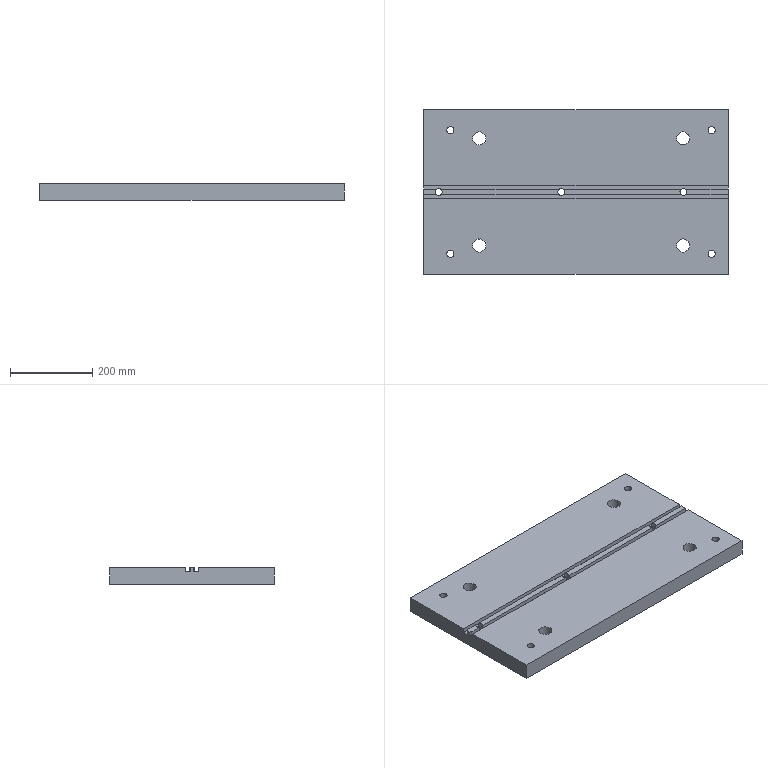Part | STEP file | lll_id5070_x_t | 1 solid | 76 faces | box 740 x 400 x 40 mm | volume 11456474 mm3 | plane 37 | cylinder 31 | cone 8 | commonest cylinder face diameters 6.806 x8 14 x4 17.506 x4 22 x4 28 x4 32 x4